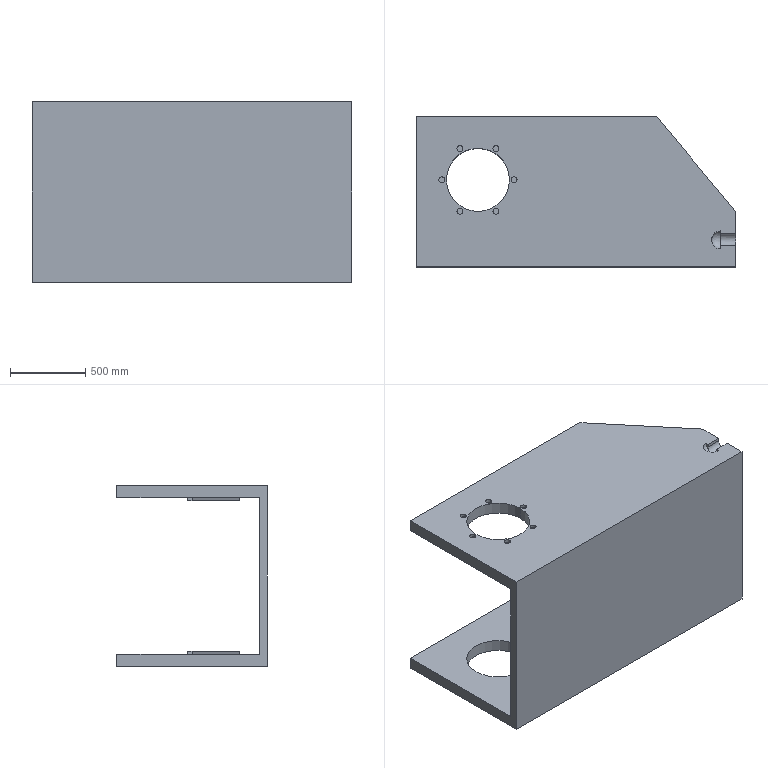Part | SolidWorks | features ICE 6, 3DProfileFeature 4, MirrorPattern 4, Extrusion 1, RevCut 1 | 1 solid | 72 faces | box 2125 x 1000 x 1200 mm | volume 401885685 mm3 | plane 40 | cylinder 30 | sphere 2 | commonest cylinder face diameters 40 x24 420 x4 80 x2